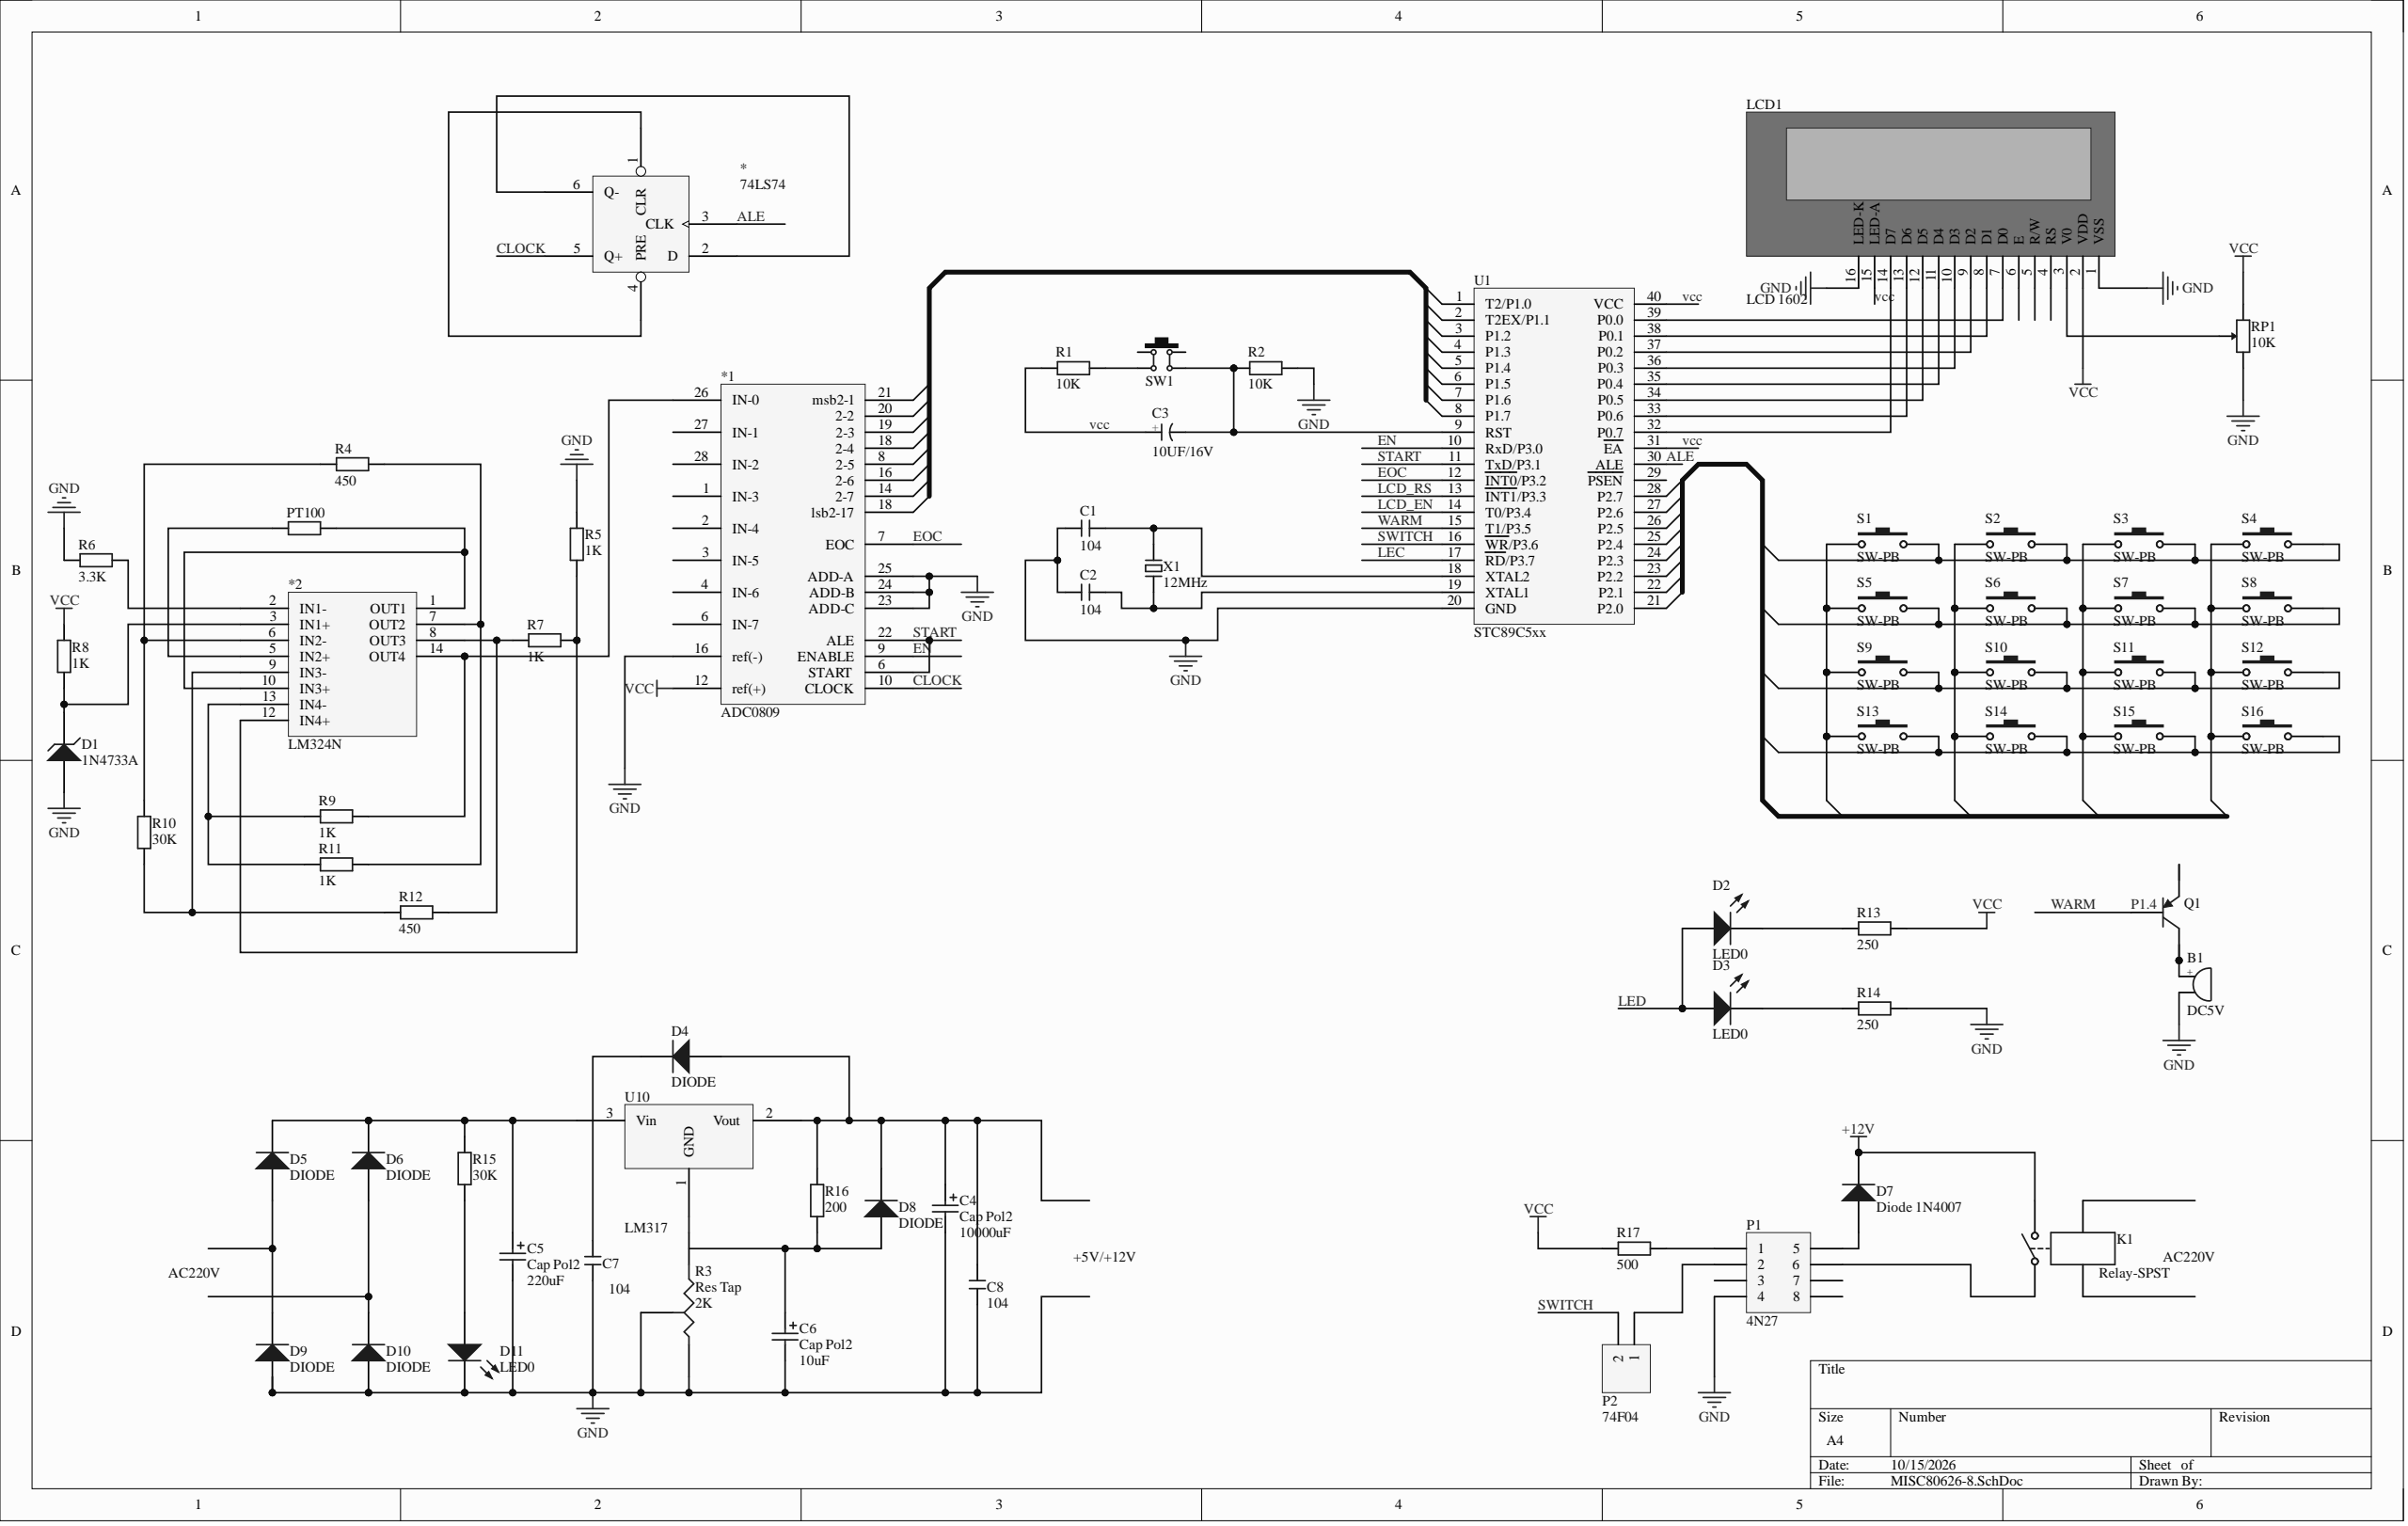Circuit board | Altium Designer | 67 parts | 60 nets
Bill of materials:
Comment,Description,Designator,Footprint,LibRef,Quantity
"74LS74","","","646-06","Component_1","1"
"ADC0809","","*1","N28B","Component_1","1"
"LM324N","","*2","646-06","Component_1","1"
"DC5V","Buzzer","B1","PIN2","BEEP","1"
"104","Through-hole ceramic capacitor","C1, C2, C7, C8","RAD-0.3","C-CC","4"
"10UF/16V","Through-hole electrolytic capacitor","C3","RB7.6-15","C-CAP","1"
"Cap Pol2","Polarized Capacitor (Axial)","C4, C5, C6","POLAR0.8","Cap Pol2","3"
"1N4733A","Zener Diode","D1","DIODE-0.7","D Zener","1"
"LED0","Typical INFRARED GaAs LED","D2, D3, D11","LED-0","LED0","3"
"DIODE","3 Amp General Purpose Rectifier","D4, D5, D6, D8, D9, D10","DO-201AD","Diode 1N5400","6"
"Diode 1N4007","3 Amp General Purpose Rectifier","D7","DO-41","Diode 1N5400","1"
"Relay-SPST","Single-Pole Single-Throw Relay","K1","MODULE4","Relay-SPST","1"
"LCD 1602","LCD 1602","LCD1","LCD1602","LCD 1602","1"
"4N27","Header, 4-Pin, Dual row","P1","HDR2X4","Header 4X2A","1"
"74F04","Header, 2-Pin","P2","HDR1X2","Header 2","1"
"30K","Through-hole colour-band resistor","PT100, R10, R15","AXIAL-0.4","R-CRR","3"
"2N3906","PNP General Purpose Amplifier","Q1","TO-92A","2N3906","1"
"10K","Through-hole colour-band resistor","R1, R2","AXIAL-0.4","R-CRR","2"
"Res Tap","Tapped Resistor","R3","VR3","Res Tap","1"
"450","Through-hole colour-band resistor","R4, R12","AXIAL-0.4","R-CRR","2"
"1K","Through-hole colour-band resistor","R5, R7, R8, R9, R11","AXIAL-0.4","R-CRR","5"
"3.3K","Through-hole colour-band resistor","R6","AXIAL-0.4","R-CRR","1"
"250","Through-hole colour-band resistor","R13, R14","AXIAL-0.4","R-CRR","2"
"200","Through-hole colour-band resistor","R16","AXIAL-0.4","R-CRR","1"
"500","Through-hole colour-band resistor","R17","AXIAL-0.4","R-CRR","1"
"10K","Plug-in single-gang potentiometer","RP1","电位器","RP-ID","1"
"SW-PB","Switch","S1, S2, S3, S4, S5, S6, S7, S8, S9, S10, S11, S12, S13, S14, S15, S16","SPST-2","SW-PB","16"
"6x6x5","Through-hole 6x6 tactile switch","SW1","四脚轻触开关","TSW DIP-6x6","1"
"STC89C5xx","STC microcontroller","U1","DIP40","STC89C5xx","1"
"LM317","Adjustable linear regulator IC","U10","TO220A","LM317","1"
"12MHz","2-pin crystal oscillator","X1","R38","XTAL-2","1"
Netlist (Protel format):
[
*
646-06
74LS74



]
[
*1
N28B
ADC0809



]
[
*2
646-06
LM324N



]
[
B1
PIN2
DC5V



]
[
C1
RAD-0.3
104



]
[
C2
RAD-0.3
104



]
[
C3
RB7.6-15
10UF/16V



]
[
C4
POLAR0.8
Cap Pol2



]
[
C5
POLAR0.8
Cap Pol2



]
[
C6
POLAR0.8
Cap Pol2



]
[
C7
RAD-0.3
104



]
[
C8
RAD-0.3
104



]
[
D1
DIODE-0.7
1N4733A



]
[
D2
LED-0
LED0



]
[
D3
LED-0
LED0



]
[
D4
DO-201AD
DIODE



]
[
D5
DO-201AD
DIODE



]
[
D6
DO-201AD
DIODE



]
[
D7
DO-41
Diode 1N4007



]
[
D8
DO-201AD
DIODE



]
[
D9
DO-201AD
DIODE



]
[
D10
DO-201AD
DIODE



]
[
D11
LED-0
LED0



]
[
K1
MODULE4
Relay-SPST



]
[
LCD1
LCD1602
LCD 1602



]
[
P1
HDR2X4
4N27



]
[
P2
HDR1X2
74F04



]
[
PT100
AXIAL-0.4
30K



]
[
Q1
TO-92A
2N3906



]
[
R1
AXIAL-0.4
10K



]
[
R2
AXIAL-0.4
10K



]
[
R3
VR3
Res Tap



]
[
R4
AXIAL-0.4
450



]
[
R5
AXIAL-0.4
1K



]
[
R6
AXIAL-0.4
3.3K



]
[
R7
AXIAL-0.4
1K



]
[
R8
AXIAL-0.4
1K



]
[
R9
AXIAL-0.4
1K



]
[
R10
AXIAL-0.4
30K



]
[
R11
AXIAL-0.4
1K



]
[
R12
AXIAL-0.4
450



]
[
R13
AXIAL-0.4
250



]
[
R14
AXIAL-0.4
250



]
[
R15
AXIAL-0.4
30K



]
[
R16
AXIAL-0.4
200



]
[
R17
AXIAL-0.4
500



]
[
RP1
电位器
10K



]
[
S1
SPST-2
SW-PB



]
[
S2
SPST-2
SW-PB



]
[
S3
SPST-2
SW-PB



]
[
S4
SPST-2
SW-PB



]
[
S5
SPST-2
SW-PB



]
[
S6
SPST-2
SW-PB



]
[
S7
SPST-2
SW-PB



]
[
S8
SPST-2
SW-PB



]
[
S9
SPST-2
SW-PB



]
[
S10
SPST-2
SW-PB



]
[
S11
SPST-2
SW-PB



]
[
S12
SPST-2
SW-PB



]
[
S13
SPST-2
SW-PB



]
[
S14
SPST-2
SW-PB



]
[
S15
SPST-2
SW-PB



]
[
S16
SPST-2
SW-PB



]
[
SW1
四脚轻触开关
6x6x5



]
[
U1
DIP40
STC89C5xx



]
[
U10
TO220A
LM317



]
[
X1
R38
12MHz



]
(
vcc
*1-12
C3-1
LCD1-2
LCD1-15
R1-1
R8-2
R13-2
R17-1
RP1-3
U1-31
U1-40
)
(
SWITCH
P2-2
U1-16
)
(
START
*1-6
*1-22
U1-11
)
(
P1.4
Q1-2
U1-15
)
(
NetS13_2
S13-2
S14-2
S15-2
S16-2
)
(
NetS9_2
S9-2
S10-2
S11-2
S12-2
)
(
NetS5_2
S5-2
S6-2
S7-2
S8-2
)
(
NetS4_1
S4-1
S8-1
S12-1
S16-1
)
(
NetS3_1
S3-1
S7-1
S11-1
S15-1
)
(
NetS2_1
S2-1
S6-1
S10-1
S14-1
)
(
NetS1_2
S1-2
S2-2
S3-2
S4-2
)
(
NetS1_1
S1-1
S5-1
S9-1
S13-1
)
(
NetR3_2
R3-2
U10-1
)
(
NetR1_2
R1-2
SW1-4
)
(
NetP1_2
P1-2
P2-1
)
(
NetP1_1
P1-1
R17-2
)
(
NetLCD1_14
LCD1-14
U1-32
)
(
NetLCD1_13
LCD1-13
U1-33
)
(
NetLCD1_12
LCD1-12
U1-34
)
(
NetLCD1_11
LCD1-11
U1-35
)
(
NetLCD1_10
LCD1-10
U1-36
)
(
NetLCD1_9
LCD1-9
U1-37
)
(
NetLCD1_8
LCD1-8
U1-38
)
(
NetLCD1_7
LCD1-7
U1-39
)
(
NetLCD1_3
LCD1-3
RP1-2
)
(
NetK1_1
K1-1
P1-6
)
(
NetD11_1
D11-1
R15-1
)
(
NetD7_1
D7-1
P1-5
)
(
NetD6_1
D6-1
D10-2
)
(
NetD5_1
D5-1
D9-2
)
(
NetD3_2
D3-2
R14-1
)
(
NetD2_2
D2-2
R13-1
)
(
NetC7_2
C7-2
D4-2
)
(
NetC6_1
C6-1
D8-1
R16-1
)
(
NetC5_1
C5-1
D5-2
D6-2
R15-2
U10-3
)
(
NetC4_1
C4-1
C8-2
D4-1
D8-2
R16-2
U10-2
)
(
NetC3_2
C3-2
R2-1
SW1-3
U1-9
)
(
NetC2_2
C2-2
U1-19
X1-1
)
(
NetC1_2
C1-2
U1-18
X1-2
)
(
NetB1_1
B1-1
Q1-3
)
(
Net*_2
*-2
*-6
)
(
Net*_1
*-1
*-4
)
(
Net*2_13
*2-13
R9-2
R11-2
)
(
Net*2_12
*2-12
R5-2
R7-1
)
(
Net*2_9
*2-9
R10-2
R12-2
)
(
Net*2_8
*2-8
R7-2
R12-1
)
(
Net*2_7
*2-7
R4-1
R11-1
)
(
Net*2_6
*2-6
R4-2
R10-1
)
(
Net*2_5
*2-5
PT100-2
)
(
Net*2_3
*2-3
D1-2
R8-1
)
(
Net*2_2
*2-2
R6-1
)
(
Net*2_1
*2-1
*2-10
PT100-1
)
(
Net*1_26
*1-26
*2-14
R9-1
)
(
LED
D2-1
D3-1
)
(
GND
*1-16
*1-23
*1-24
*1-25
B1-2
C1-1
C2-1
C4-2
C5-2
C6-2
C7-1
C8-1
D1-1
D9-1
D10-1
D11-2
LCD1-1
LCD1-16
P1-4
R2-2
R3-1
R3-3
R5-1
R6-2
R14-2
RP1-1
U1-20
)
(
EOC
*1-7
U1-12
)
(
EN
*1-9
U1-10
)
(
CLOCK
*-5
*1-10
)
(
ALE
*-3
U1-30
)
(
+12V
D7-2
K1-2
)